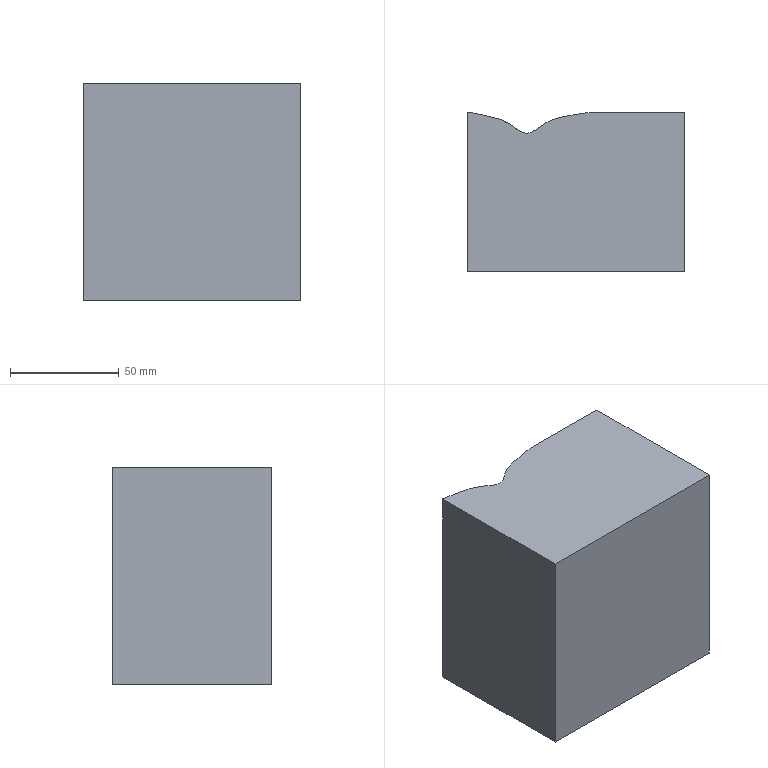Part | NX | features solid 2 | 1 solid | 6 faces | box 100 x 73.227 x 100 mm | volume 707404 mm3 | plane 5 | spline 1
STEP:
#1=CARTESIAN_POINT('',(140.,603.075,250.));
#2=VERTEX_POINT('',#1);
#3=CARTESIAN_POINT('',(140.,603.075,150.));
#4=VERTEX_POINT('',#3);
#5=CARTESIAN_POINT('',(140.,603.075,200.));
#6=DIRECTION('',(0.,0.,1.));
#7=VECTOR('',#6,1000.);
#8=LINE('',#5,#7);
#9=EDGE_CURVE('',#2,#4,#8,.F.);
#10=ORIENTED_EDGE('',*,*,#9,.F.);
#11=CARTESIAN_POINT('',(140.,530.,250.));
#12=VERTEX_POINT('',#11);
#13=CARTESIAN_POINT('',(140.,540.,250.));
#14=DIRECTION('',(0.,-1.,0.));
#15=VECTOR('',#14,1000.);
#16=LINE('',#13,#15);
#17=EDGE_CURVE('',#2,#12,#16,.T.);
#18=ORIENTED_EDGE('',*,*,#17,.T.);
#19=CARTESIAN_POINT('',(140.,530.,150.));
#20=VERTEX_POINT('',#19);
#21=CARTESIAN_POINT('',(140.,530.,250.));
#22=DIRECTION('',(0.,0.,-1.));
#23=VECTOR('',#22,1000.);
#24=LINE('',#21,#23);
#25=EDGE_CURVE('',#12,#20,#24,.T.);
#26=ORIENTED_EDGE('',*,*,#25,.T.);
#27=CARTESIAN_POINT('',(140.,540.,150.));
#28=DIRECTION('',(0.,-1.,0.));
#29=VECTOR('',#28,1000.);
#30=LINE('',#27,#29);
#31=EDGE_CURVE('',#4,#20,#30,.T.);
#32=ORIENTED_EDGE('',*,*,#31,.F.);
#33=EDGE_LOOP('',(#10,#18,#26,#32));
#34=FACE_BOUND('',#33,.T.);
#35=CARTESIAN_POINT('',(140.,540.,250.));
#36=DIRECTION('',(1.,0.,0.));
#37=DIRECTION('',(0.,0.,-1.));
#38=AXIS2_PLACEMENT_3D('',#35,#36,#37);
#39=PLANE('',#38);
#40=ADVANCED_FACE('',(#34),#39,.T.);
#41=CARTESIAN_POINT('',(40.,603.182,150.));
#42=VERTEX_POINT('',#41);
#43=CARTESIAN_POINT('',(140.,603.075,150.));
#44=CARTESIAN_POINT('',(135.738,603.019,150.));
#45=CARTESIAN_POINT('',(127.2,603.173,150.));
#46=CARTESIAN_POINT('',(116.539,603.145,150.));
#47=CARTESIAN_POINT('',(108.007,603.182,150.));
#48=CARTESIAN_POINT('',(101.606,603.258,150.));
#49=CARTESIAN_POINT('',(95.217,603.106,150.));
#50=CARTESIAN_POINT('',(89.94,602.145,150.));
#51=CARTESIAN_POINT('',(85.721,601.32,150.));
#52=CARTESIAN_POINT('',(82.558,600.755,150.));
#53=CARTESIAN_POINT('',(79.388,599.968,150.));
#54=CARTESIAN_POINT('',(76.33,598.515,150.));
#55=CARTESIAN_POINT('',(73.631,596.577,150.));
#56=CARTESIAN_POINT('',(70.995,594.554,150.));
#57=CARTESIAN_POINT('',(68.408,593.34,150.));
#58=CARTESIAN_POINT('',(66.153,593.555,150.));
#59=CARTESIAN_POINT('',(64.105,594.432,150.));
#60=CARTESIAN_POINT('',(61.863,596.072,150.));
#61=CARTESIAN_POINT('',(59.196,598.054,150.));
#62=CARTESIAN_POINT('',(56.307,599.614,150.));
#63=CARTESIAN_POINT('',(53.107,600.614,150.));
#64=CARTESIAN_POINT('',(49.842,601.317,150.));
#65=CARTESIAN_POINT('',(45.495,602.277,150.));
#66=CARTESIAN_POINT('',(42.221,602.931,150.));
#67=CARTESIAN_POINT('',(40.,603.182,150.));
#68=B_SPLINE_CURVE_WITH_KNOTS('',3,(#43,#44,#45,#46,#47,#48,#49,#50,#51,#52,#53,#54,#55,#56,#57,#58,#59,#60,#61,#62,#63,#64,#65,#66,#67),.UNSPECIFIED.,.F.,.F.,(4,1,1,1,1,1,1,1,1,1,1,1,1,1,1,1,1,1,1,1,1,1,4),(0.,0.01277,0.02555,0.03194,0.03832,0.04471,0.0511,0.05429,0.05748,0.06068,0.06387,0.06707,0.07026,0.07345,0.07505,0.07665,0.07984,0.08303,0.08623,0.08942,0.09261,0.09581,0.1022),.UNSPECIFIED.);
#69=EDGE_CURVE('',#4,#42,#68,.T.);
#70=ORIENTED_EDGE('',*,*,#69,.F.);
#71=ORIENTED_EDGE('',*,*,#31,.T.);
#72=CARTESIAN_POINT('',(40.,530.,150.));
#73=VERTEX_POINT('',#72);
#74=CARTESIAN_POINT('',(140.,530.,150.));
#75=DIRECTION('',(-1.,0.,0.));
#76=VECTOR('',#75,1000.);
#77=LINE('',#74,#76);
#78=EDGE_CURVE('',#20,#73,#77,.T.);
#79=ORIENTED_EDGE('',*,*,#78,.T.);
#80=CARTESIAN_POINT('',(40.,540.,150.));
#81=DIRECTION('',(0.,-1.,0.));
#82=VECTOR('',#81,1000.);
#83=LINE('',#80,#82);
#84=EDGE_CURVE('',#42,#73,#83,.T.);
#85=ORIENTED_EDGE('',*,*,#84,.F.);
#86=EDGE_LOOP('',(#70,#71,#79,#85));
#87=FACE_BOUND('',#86,.T.);
#88=CARTESIAN_POINT('',(140.,540.,150.));
#89=DIRECTION('',(0.,0.,-1.));
#90=DIRECTION('',(-1.,0.,0.));
#91=AXIS2_PLACEMENT_3D('',#88,#89,#90);
#92=PLANE('',#91);
#93=ADVANCED_FACE('',(#87),#92,.T.);
#94=CARTESIAN_POINT('',(40.,603.182,250.));
#95=VERTEX_POINT('',#94);
#96=CARTESIAN_POINT('',(40.,603.182,250.));
#97=CARTESIAN_POINT('',(42.158,602.938,250.));
#98=CARTESIAN_POINT('',(45.34,602.311,250.));
#99=CARTESIAN_POINT('',(49.565,601.377,250.));
#100=CARTESIAN_POINT('',(52.733,600.699,250.));
#101=CARTESIAN_POINT('',(55.871,599.782,250.));
#102=CARTESIAN_POINT('',(58.734,598.347,250.));
#103=CARTESIAN_POINT('',(61.371,596.458,250.));
#104=CARTESIAN_POINT('',(63.934,594.508,250.));
#105=CARTESIAN_POINT('',(66.998,593.097,250.));
#106=CARTESIAN_POINT('',(70.256,594.053,250.));
#107=CARTESIAN_POINT('',(72.839,595.964,250.));
#108=CARTESIAN_POINT('',(75.434,597.912,250.));
#109=CARTESIAN_POINT('',(78.215,599.504,250.));
#110=CARTESIAN_POINT('',(81.358,600.512,250.));
#111=CARTESIAN_POINT('',(84.56,601.111,250.));
#112=CARTESIAN_POINT('',(88.826,601.911,250.));
#113=CARTESIAN_POINT('',(94.151,602.987,250.));
#114=CARTESIAN_POINT('',(100.664,603.277,250.));
#115=CARTESIAN_POINT('',(107.226,603.183,250.));
#116=CARTESIAN_POINT('',(115.964,603.15,250.));
#117=CARTESIAN_POINT('',(126.89,603.174,250.));
#118=CARTESIAN_POINT('',(135.63,603.017,250.));
#119=CARTESIAN_POINT('',(140.,603.075,250.));
#120=B_SPLINE_CURVE_WITH_KNOTS('',3,(#96,#97,#98,#99,#100,#101,#102,#103,#104,#105,#106,#107,#108,#109,#110,#111,#112,#113,#114,#115,#116,#117,#118,#119),.UNSPECIFIED.,.F.,.F.,(4,1,1,1,1,1,1,1,1,1,1,1,1,1,1,1,1,1,1,1,1,4),(0.,0.006488,0.009731,0.01298,0.01622,0.01946,0.02271,0.02595,0.02919,0.03244,0.03568,0.03893,0.04217,0.04541,0.04866,0.0519,0.05839,0.06488,0.07136,0.07785,0.09083,0.1038),.UNSPECIFIED.);
#121=EDGE_CURVE('',#95,#2,#120,.T.);
#122=ORIENTED_EDGE('',*,*,#121,.F.);
#123=CARTESIAN_POINT('',(40.,530.,250.));
#124=VERTEX_POINT('',#123);
#125=CARTESIAN_POINT('',(40.,540.,250.));
#126=DIRECTION('',(0.,-1.,0.));
#127=VECTOR('',#126,1000.);
#128=LINE('',#125,#127);
#129=EDGE_CURVE('',#95,#124,#128,.T.);
#130=ORIENTED_EDGE('',*,*,#129,.T.);
#131=CARTESIAN_POINT('',(40.,530.,250.));
#132=DIRECTION('',(1.,0.,0.));
#133=VECTOR('',#132,1000.);
#134=LINE('',#131,#133);
#135=EDGE_CURVE('',#124,#12,#134,.T.);
#136=ORIENTED_EDGE('',*,*,#135,.T.);
#137=ORIENTED_EDGE('',*,*,#17,.F.);
#138=EDGE_LOOP('',(#122,#130,#136,#137));
#139=FACE_BOUND('',#138,.T.);
#140=CARTESIAN_POINT('',(40.,540.,250.));
#141=DIRECTION('',(0.,0.,1.));
#142=DIRECTION('',(0.,1.,0.));
#143=AXIS2_PLACEMENT_3D('',#140,#141,#142);
#144=PLANE('',#143);
#145=ADVANCED_FACE('',(#139),#144,.T.);
#146=ORIENTED_EDGE('',*,*,#135,.F.);
#147=CARTESIAN_POINT('',(40.,530.,150.));
#148=DIRECTION('',(0.,0.,1.));
#149=VECTOR('',#148,1000.);
#150=LINE('',#147,#149);
#151=EDGE_CURVE('',#73,#124,#150,.T.);
#152=ORIENTED_EDGE('',*,*,#151,.F.);
#153=ORIENTED_EDGE('',*,*,#78,.F.);
#154=ORIENTED_EDGE('',*,*,#25,.F.);
#155=EDGE_LOOP('',(#146,#152,#153,#154));
#156=FACE_BOUND('',#155,.T.);
#157=CARTESIAN_POINT('',(140.,530.,150.));
#158=DIRECTION('',(0.,-1.,0.));
#159=DIRECTION('',(0.,0.,1.));
#160=AXIS2_PLACEMENT_3D('',#157,#158,#159);
#161=PLANE('',#160);
#162=ADVANCED_FACE('',(#156),#161,.T.);
#163=CARTESIAN_POINT('',(40.,603.182,200.));
#164=DIRECTION('',(0.,0.,1.));
#165=VECTOR('',#164,1000.);
#166=LINE('',#163,#165);
#167=EDGE_CURVE('',#42,#95,#166,.T.);
#168=ORIENTED_EDGE('',*,*,#167,.F.);
#169=ORIENTED_EDGE('',*,*,#84,.T.);
#170=ORIENTED_EDGE('',*,*,#151,.T.);
#171=ORIENTED_EDGE('',*,*,#129,.F.);
#172=EDGE_LOOP('',(#168,#169,#170,#171));
#173=FACE_BOUND('',#172,.T.);
#174=CARTESIAN_POINT('',(40.,540.,150.));
#175=DIRECTION('',(-1.,0.,0.));
#176=DIRECTION('',(0.,1.,0.));
#177=AXIS2_PLACEMENT_3D('',#174,#175,#176);
#178=PLANE('',#177);
#179=ADVANCED_FACE('',(#173),#178,.T.);
#180=ORIENTED_EDGE('',*,*,#121,.T.);
#181=ORIENTED_EDGE('',*,*,#9,.T.);
#182=ORIENTED_EDGE('',*,*,#69,.T.);
#183=ORIENTED_EDGE('',*,*,#167,.T.);
#184=EDGE_LOOP('',(#180,#181,#182,#183));
#185=FACE_BOUND('',#184,.T.);
#186=CARTESIAN_POINT('',(140.,603.075,150.));
#187=CARTESIAN_POINT('',(140.,603.075,250.));
#188=CARTESIAN_POINT('',(135.667,603.018,150.));
#189=CARTESIAN_POINT('',(135.667,603.018,250.));
#190=CARTESIAN_POINT('',(126.994,603.173,150.));
#191=CARTESIAN_POINT('',(126.994,603.173,250.));
#192=CARTESIAN_POINT('',(116.157,603.148,150.));
#193=CARTESIAN_POINT('',(116.157,603.148,250.));
#194=CARTESIAN_POINT('',(107.489,603.183,150.));
#195=CARTESIAN_POINT('',(107.489,603.183,250.));
#196=CARTESIAN_POINT('',(100.985,603.271,150.));
#197=CARTESIAN_POINT('',(100.985,603.271,250.));
#198=CARTESIAN_POINT('',(94.487,603.031,150.));
#199=CARTESIAN_POINT('',(94.487,603.031,250.));
#200=CARTESIAN_POINT('',(89.118,601.972,150.));
#201=CARTESIAN_POINT('',(89.118,601.972,250.));
#202=CARTESIAN_POINT('',(84.881,601.169,150.));
#203=CARTESIAN_POINT('',(84.881,601.169,250.));
#204=CARTESIAN_POINT('',(81.745,600.591,150.));
#205=CARTESIAN_POINT('',(81.745,600.591,250.));
#206=CARTESIAN_POINT('',(78.672,599.697,150.));
#207=CARTESIAN_POINT('',(78.672,599.697,250.));
#208=CARTESIAN_POINT('',(75.68,598.107,150.));
#209=CARTESIAN_POINT('',(75.68,598.107,250.));
#210=CARTESIAN_POINT('',(72.778,595.897,150.));
#211=CARTESIAN_POINT('',(72.778,595.897,250.));
#212=CARTESIAN_POINT('',(69.957,593.912,150.));
#213=CARTESIAN_POINT('',(69.957,593.912,250.));
#214=CARTESIAN_POINT('',(67.188,593.198,150.));
#215=CARTESIAN_POINT('',(67.188,593.198,250.));
#216=CARTESIAN_POINT('',(64.432,594.184,150.));
#217=CARTESIAN_POINT('',(64.432,594.184,250.));
#218=CARTESIAN_POINT('',(61.639,596.243,150.));
#219=CARTESIAN_POINT('',(61.639,596.243,250.));
#220=CARTESIAN_POINT('',(57.806,599.061,150.));
#221=CARTESIAN_POINT('',(57.806,599.061,250.));
#222=CARTESIAN_POINT('',(53.769,600.488,150.));
#223=CARTESIAN_POINT('',(53.769,600.488,250.));
#224=CARTESIAN_POINT('',(49.598,601.368,150.));
#225=CARTESIAN_POINT('',(49.598,601.368,250.));
#226=CARTESIAN_POINT('',(45.372,602.306,150.));
#227=CARTESIAN_POINT('',(45.372,602.306,250.));
#228=CARTESIAN_POINT('',(42.156,602.938,150.));
#229=CARTESIAN_POINT('',(42.156,602.938,250.));
#230=CARTESIAN_POINT('',(40.,603.182,150.));
#231=CARTESIAN_POINT('',(40.,603.182,250.));
#232=B_SPLINE_SURFACE_WITH_KNOTS('',3,1,((#186,#187),(#188,#189),(#190,#191),(#192,#193),(#194,#195),(#196,#197),(#198,#199),(#200,#201),(#202,#203),(#204,#205),(#206,#207),(#208,#209),(#210,#211),(#212,#213),(#214,#215),(#216,#217),(#218,#219),(#220,#221),(#222,#223),(#224,#225),(#226,#227),(#228,#229),(#230,#231)),.SURF_OF_LINEAR_EXTRUSION.,.F.,.F.,.F.,(4,1,1,1,1,1,1,1,1,1,1,1,1,1,1,1,1,1,1,1,4),(2,2),(0.1885,0.1905,0.1925,0.1935,0.1945,0.1956,0.1966,0.1971,0.1976,0.1981,0.1986,0.1991,0.1996,0.2001,0.2006,0.2011,0.2016,0.2026,0.2031,0.2036,0.2046),(0.,1.),.UNSPECIFIED.);
#233=ADVANCED_FACE('',(#185),#232,.T.);
#234=CLOSED_SHELL('',(#40,#93,#145,#162,#179,#233));
#235=MANIFOLD_SOLID_BREP('',#234);
#236=(LENGTH_UNIT()NAMED_UNIT(*)SI_UNIT(.MILLI.,.METRE.));
#237=UNCERTAINTY_MEASURE_WITH_UNIT(LENGTH_MEASURE(0.0508),#236,'','');
#238=(NAMED_UNIT(*)PLANE_ANGLE_UNIT()SI_UNIT($,.RADIAN.));
#239=(NAMED_UNIT(*)SI_UNIT($,.STERADIAN.)SOLID_ANGLE_UNIT());
#240=(GEOMETRIC_REPRESENTATION_CONTEXT(3)GLOBAL_UNCERTAINTY_ASSIGNED_CONTEXT((#237))GLOBAL_UNIT_ASSIGNED_CONTEXT((#236,#238,#239))REPRESENTATION_CONTEXT('',''));
#241=ADVANCED_BREP_SHAPE_REPRESENTATION('',(#235),#240);